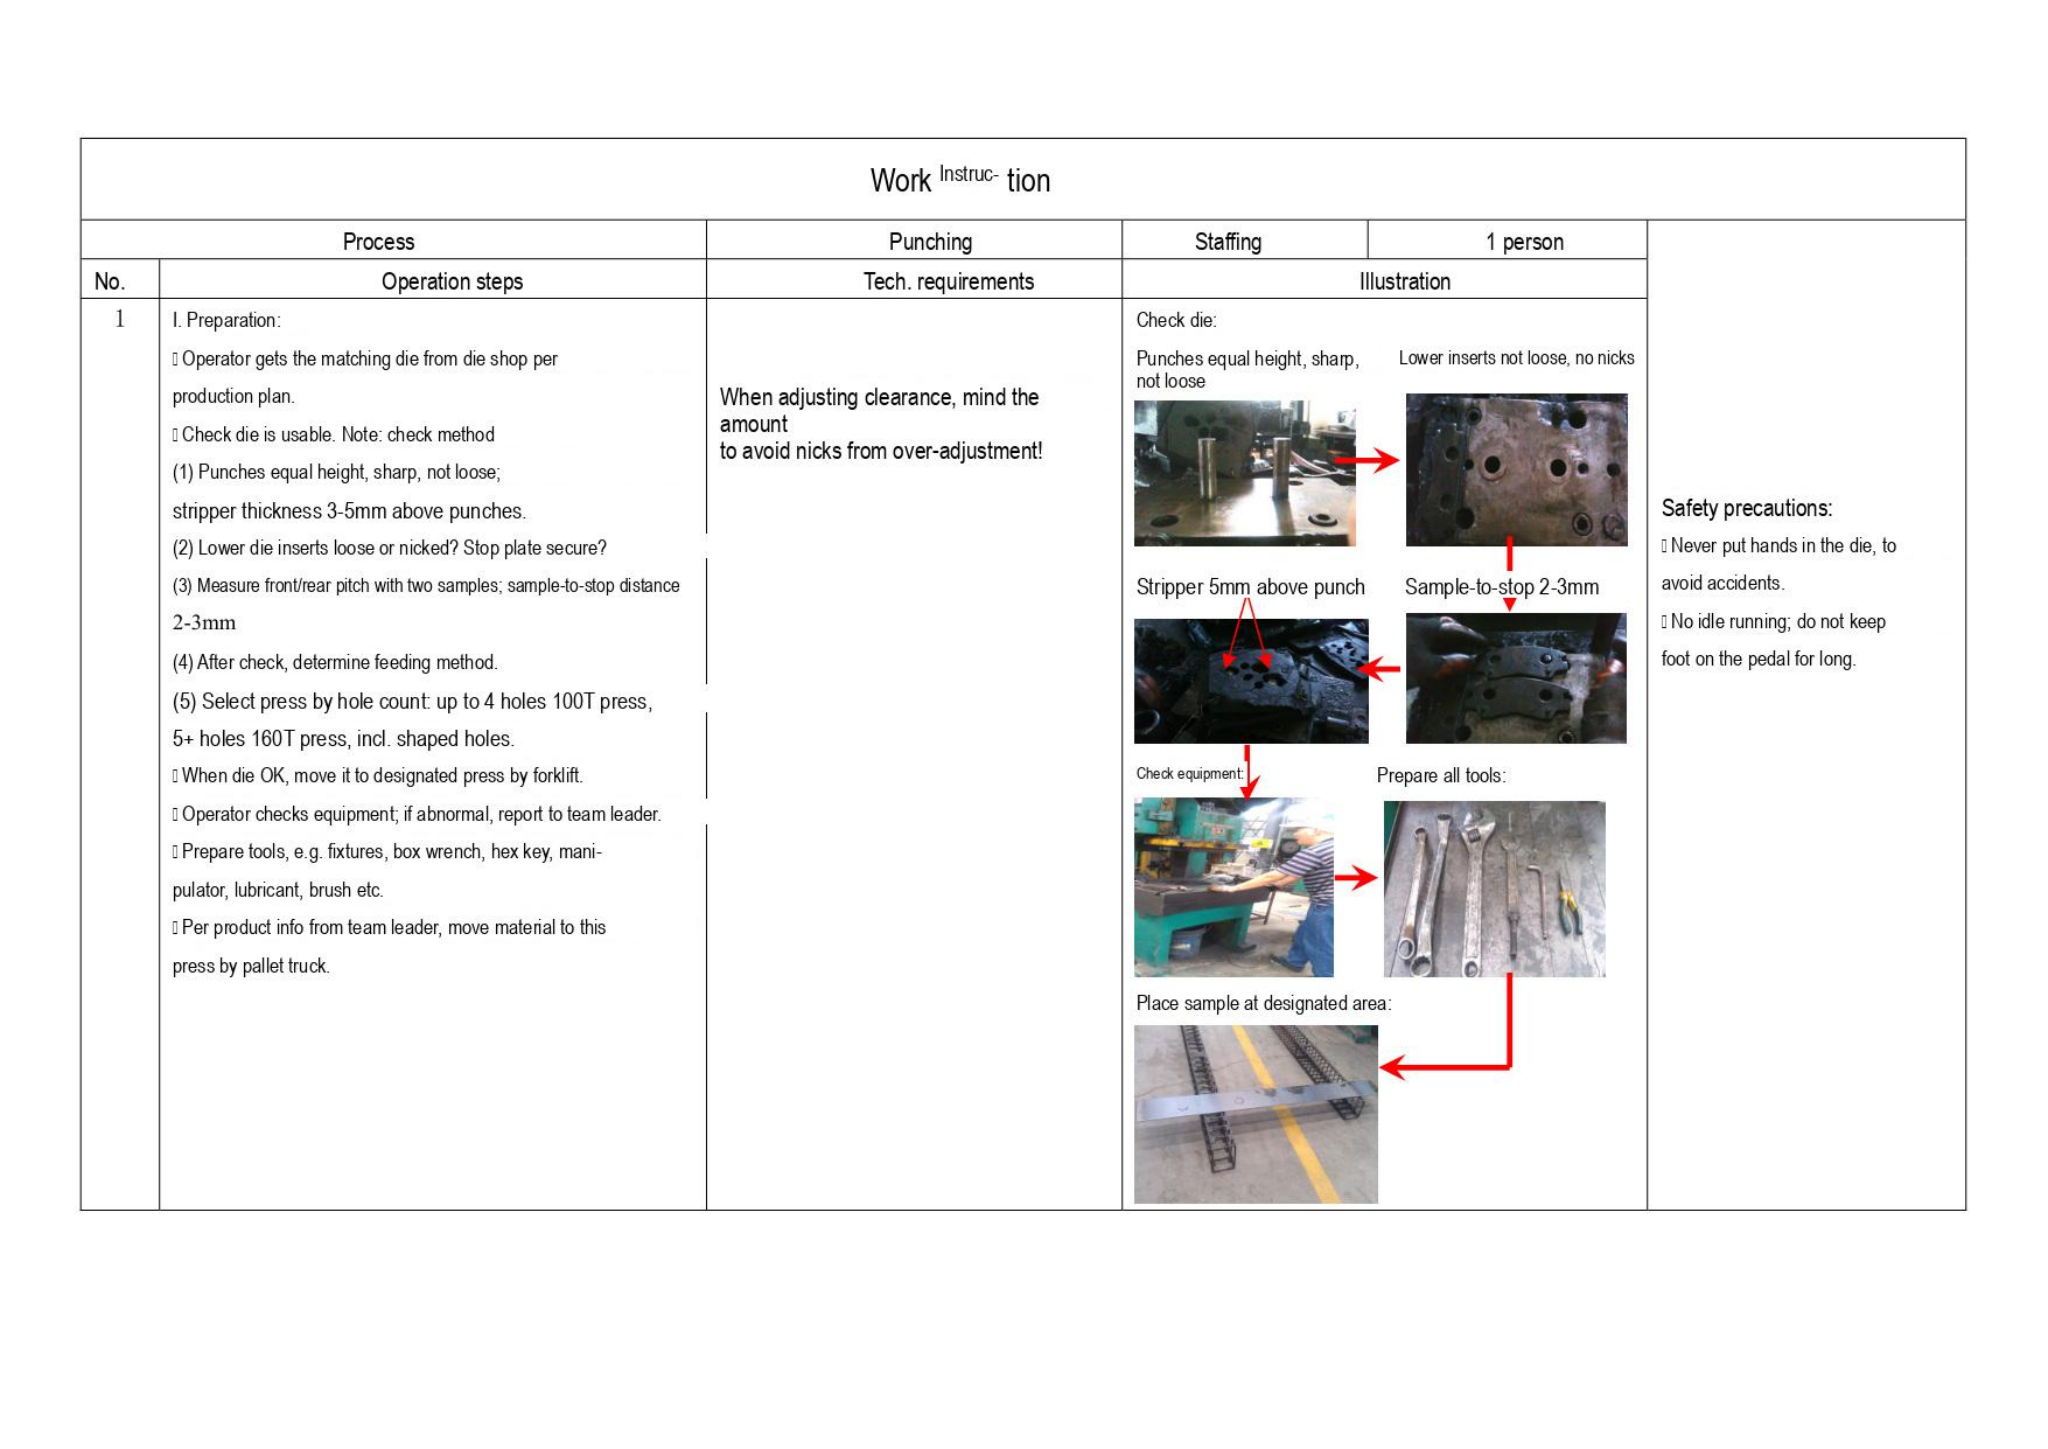Work Instruc- tion

| Process | | Punching | Staffing | 1 person | |
|---|---|---|---|---|---|
| No. | Operation steps | Tech. requirements | Illustration | | |
| 1 | I. Preparation:<br>▯ Operator gets the matching die from die shop per production plan.<br>▯ Check die is usable. Note: check method<br>(1) Punches equal height, sharp, not loose;<br>stripper thickness 3-5mm above punches.<br>(2) Lower die inserts loose or nicked? Stop plate secure?<br>(3) Measure front/rear pitch with two samples; sample-to-stop distance 2-3mm<br>(4) After check, determine feeding method.<br>(5) Select press by hole count: up to 4 holes 100T press, 5+ holes 160T press, incl. shaped holes.<br>▯ When die OK, move it to designated press by forklift.<br>▯ Operator checks equipment; if abnormal, report to team leader.<br>▯ Prepare tools, e.g. fixtures, box wrench, hex key, manipulator, lubricant, brush etc.<br>▯ Per product info from team leader, move material to this press by pallet truck. | When adjusting clearance, mind the amount<br>to avoid nicks from over-adjustment! | Check die:<br>Punches equal height, sharp, not loose<br>Lower inserts not loose, no nicks<br>Stripper 5mm above punch<br>Sample-to-stop 2-3mm<br>Check equipment:<br>Prepare all tools:<br>Place sample at designated area: | | Safety precautions:<br>▯ Never put hands in the die, to avoid accidents.<br>▯ No idle running; do not keep foot on the pedal for long. |
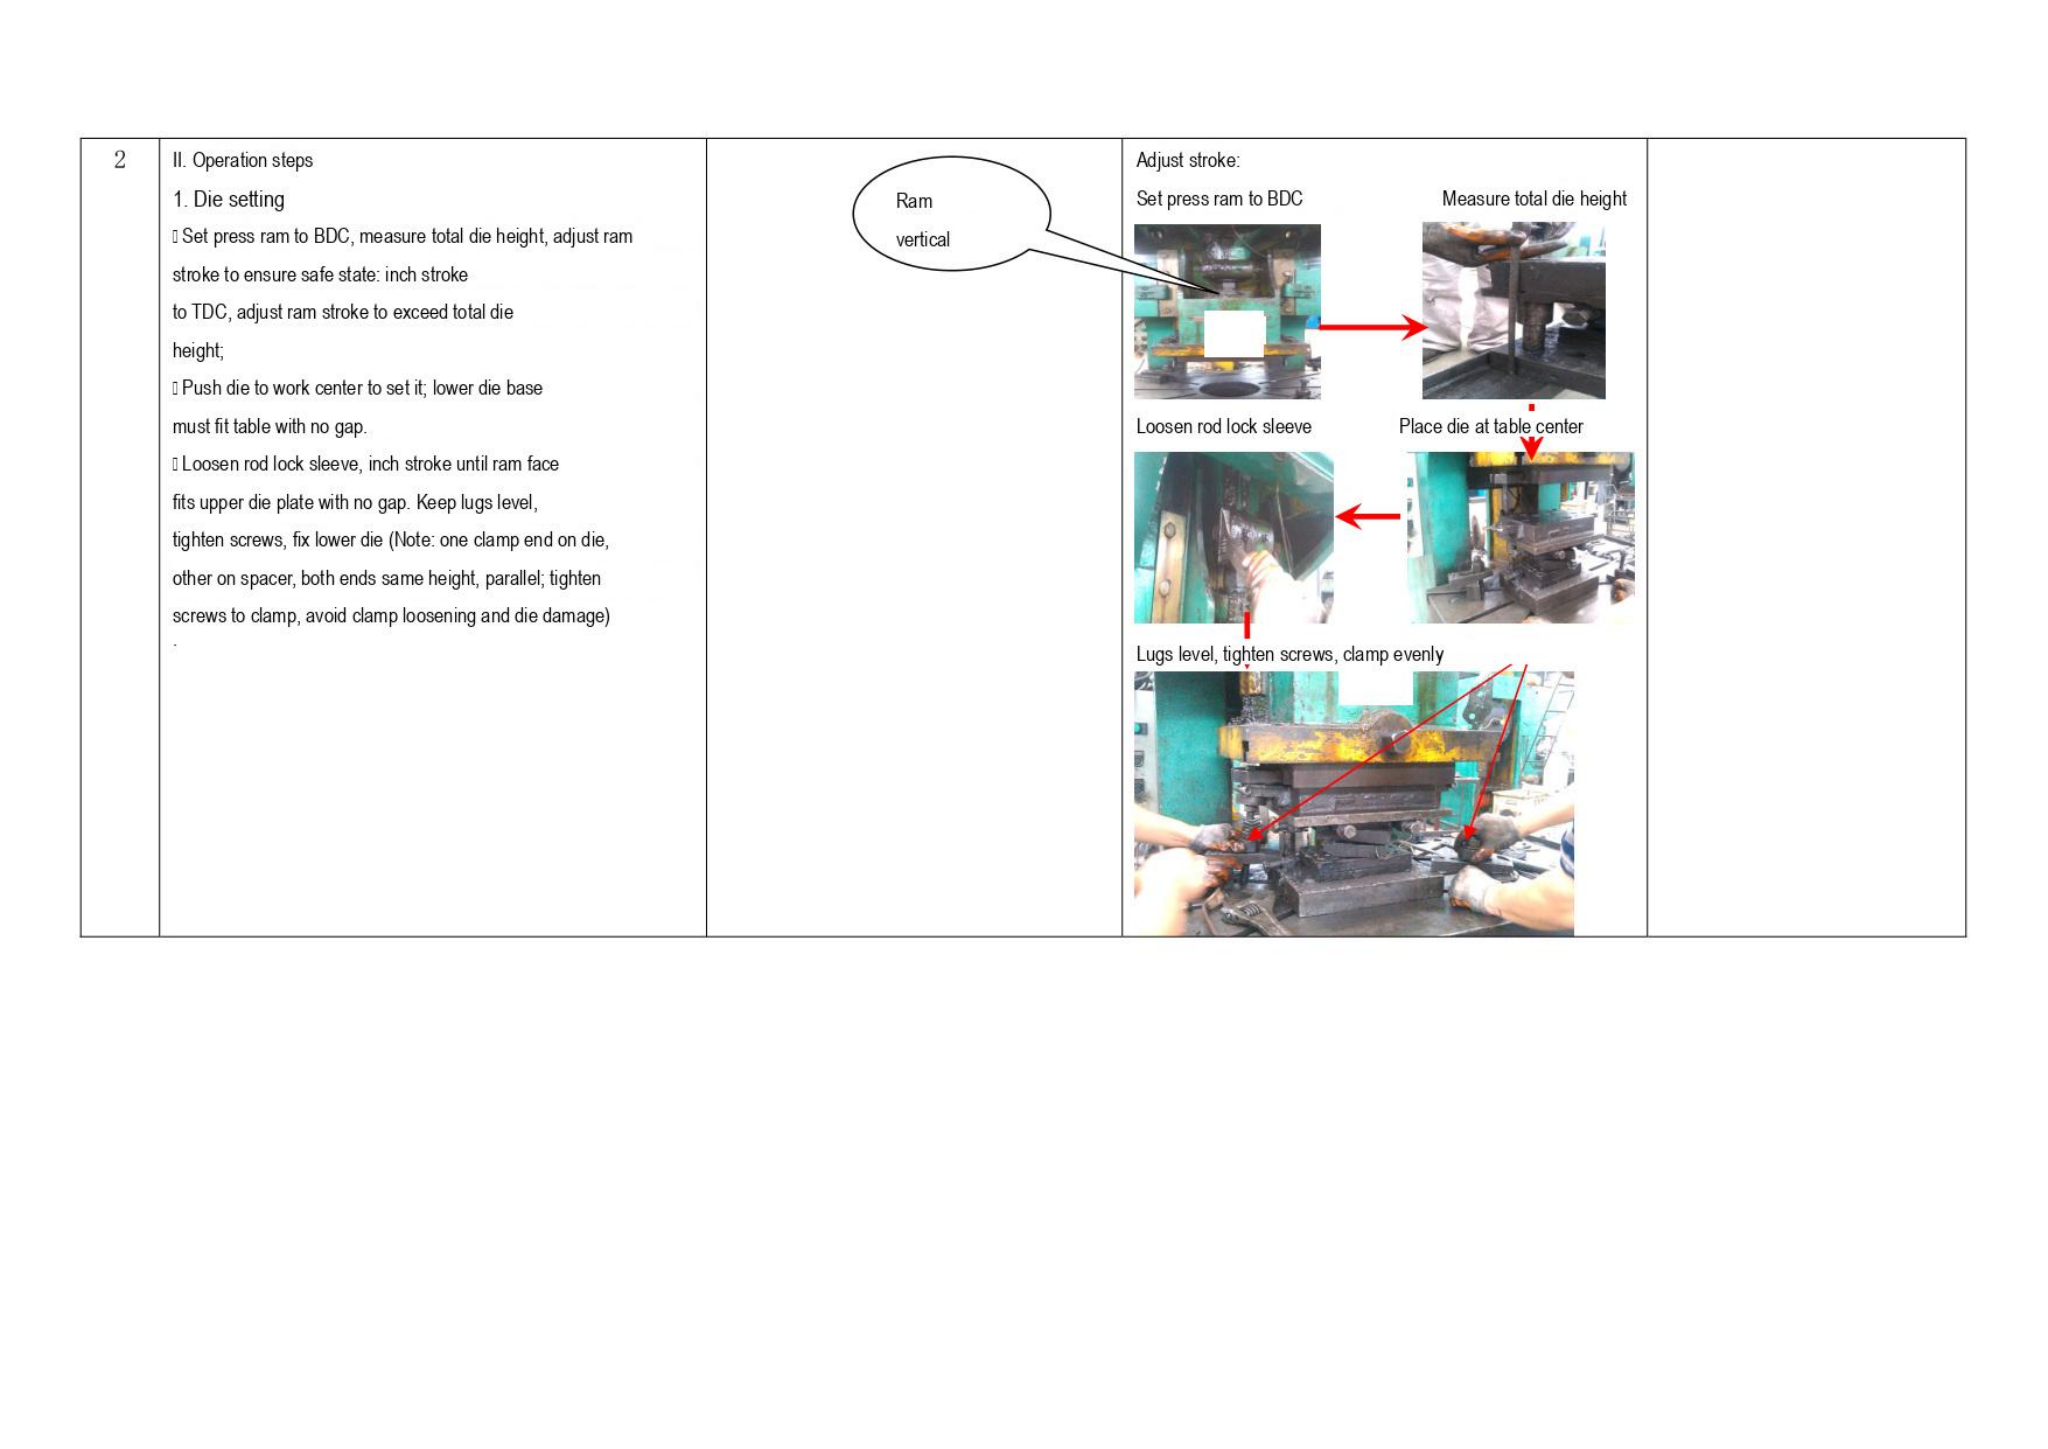| 2 | II. Operation steps<br>1. Die setting<br>Set press ram to BDC, measure total die height, adjust ram stroke to ensure safe state: inch stroke to TDC, adjust ram stroke to exceed total die height;<br>Push die to work center to set it; lower die base must fit table with no gap.<br>Loosen rod lock sleeve, inch stroke until ram face fits upper die plate with no gap. Keep lugs level, tighten screws, fix lower die (Note: one clamp end on die, other on spacer, both ends same height, parallel; tighten screws to clamp, avoid clamp loosening and die damage) | Ram vertical | Adjust stroke:<br>Set press ram to BDC<br>Measure total die height<br>Loosen rod lock sleeve<br>Place die at table center<br>Lugs level, tighten screws, clamp evenly | |
|---|---|---|---|---|
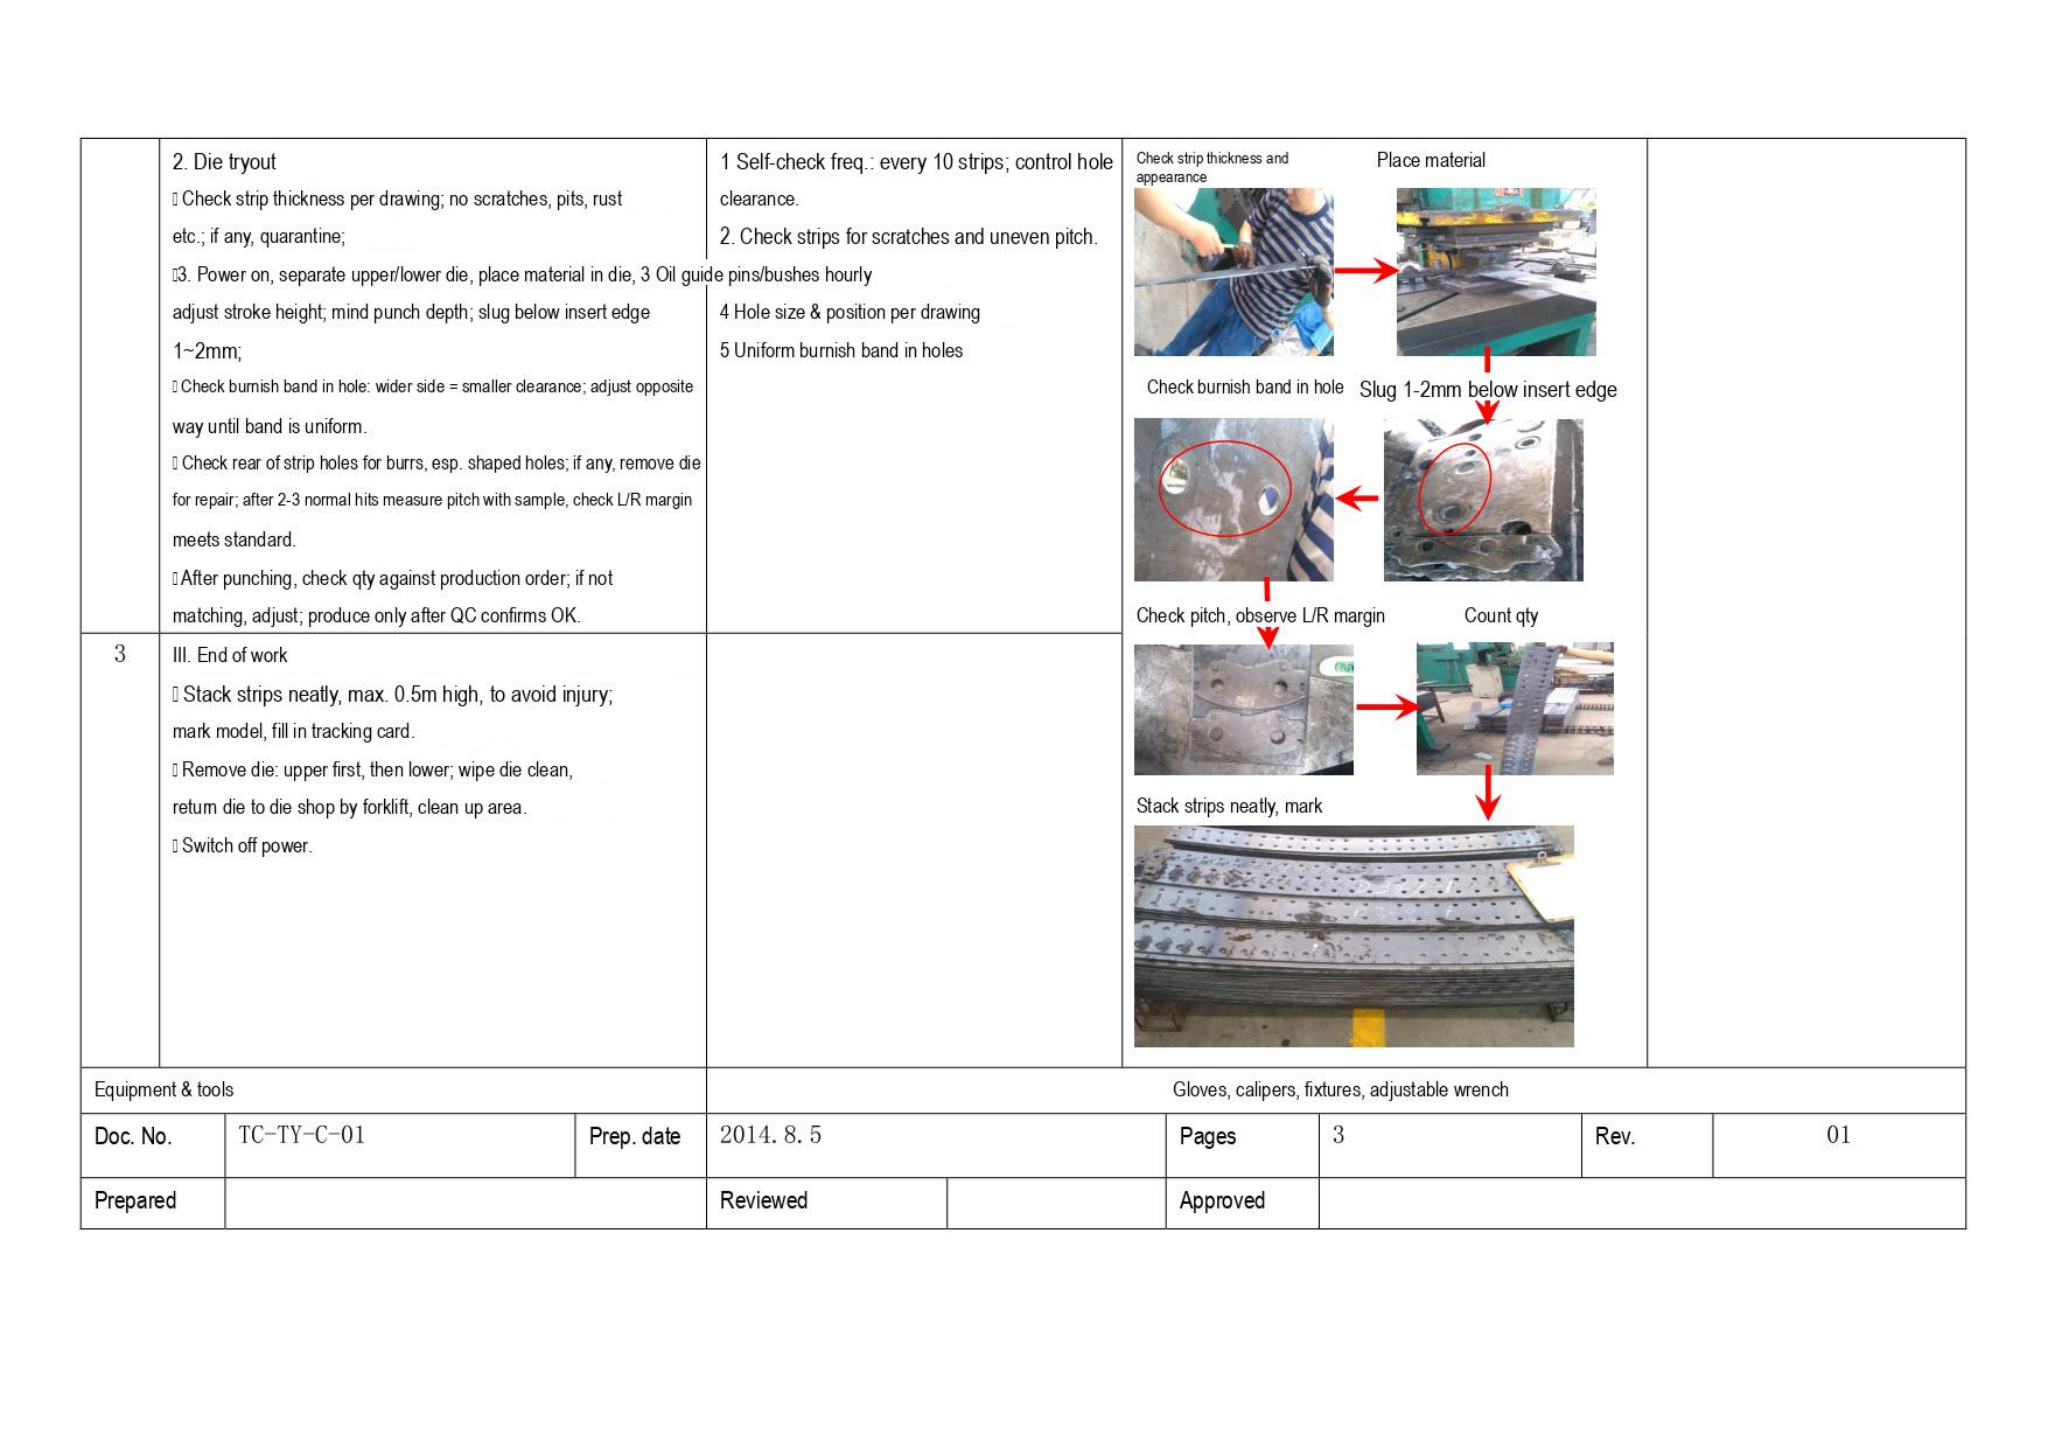| | 2. Die tryout<br>Check strip thickness per drawing; no scratches, pits, rust etc.; if any, quarantine;<br>3. Power on, separate upper/lower die, place material in die, adjust stroke height; mind punch depth; slug below insert edge 1~2mm;<br>Check burnish band in hole: wider side = smaller clearance; adjust opposite way until band is uniform.<br>Check rear of strip holes for burrs, esp. shaped holes; if any, remove die for repair; after 2-3 normal hits measure pitch with sample, check L/R margin meets standard.<br>After punching, check qty against production order; if not matching, adjust; produce only after QC confirms OK. | 1 Self-check freq.: every 10 strips; control hole clearance.<br>2. Check strips for scratches and uneven pitch.<br>3 Oil guide pins/bushes hourly<br>4 Hole size & position per drawing<br>5 Uniform burnish band in holes | Check strip thickness and appearance<br>Place material<br>Check burnish band in hole<br>Slug 1-2mm below insert edge<br>Check pitch, observe L/R margin<br>Count qty<br>Stack strips neatly, mark | |
|---|---|---|---|---|
| 3 | III. End of work<br>Stack strips neatly, max. 0.5m high, to avoid injury; mark model, fill in tracking card.<br>Remove die: upper first, then lower; wipe die clean, return die to die shop by forklift, clean up area.<br>Switch off power. | | | |

| Equipment & tools | Gloves, calipers, fixtures, adjustable wrench |
|---|---|

| Doc. No. | TC-TY-C-01 | Prep. date | 2014. 8. 5 | Pages | 3 | Rev. | 01 |
|---|---|---|---|---|---|---|---|
| Prepared | | Reviewed | | Approved | | | |